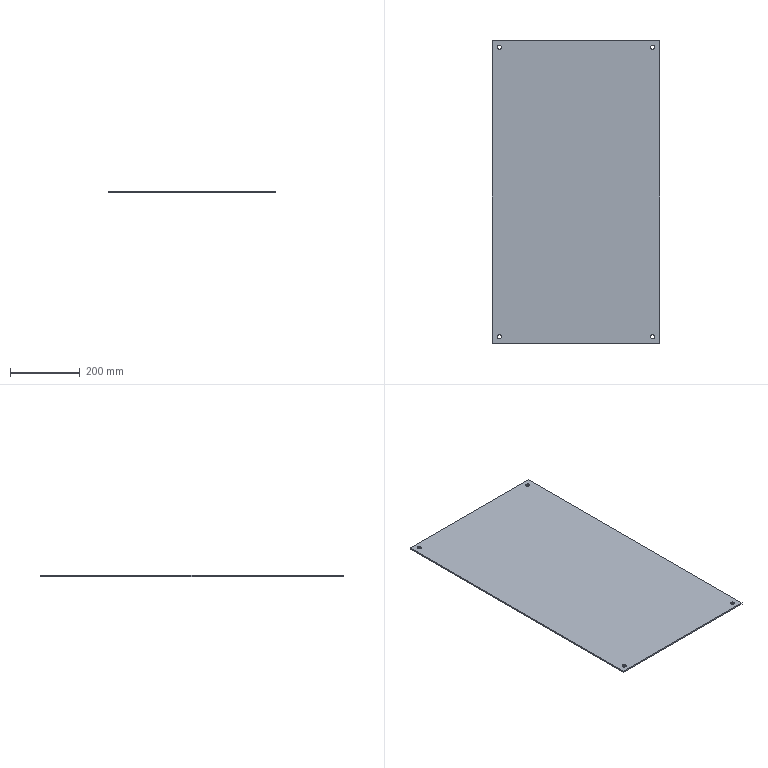Part | STEP file | 02 Middle cover plate | 1 solid | 14 faces | box 480 x 866 x 4 mm | volume 1660910 mm3 | cylinder 8 | plane 6 | commonest cylinder face diameters 12 x8
STEP:
#1=CARTESIAN_POINT('',(0.,0.,0.));
#2=DIRECTION('',(0.,0.,1.));
#3=DIRECTION('',(1.,0.,0.));
#4=AXIS2_PLACEMENT_3D('',#1,#2,#3);
#5=CARTESIAN_POINT('',(14.,-18.,4.));
#6=VERTEX_POINT('',#5);
#7=CARTESIAN_POINT('',(14.,-18.,0.));
#8=VERTEX_POINT('',#7);
#9=CARTESIAN_POINT('',(14.,-18.,4.));
#10=DIRECTION('',(0.,0.,-1.));
#11=VECTOR('',#10,1.);
#12=LINE('',#9,#11);
#13=CARTESIAN_POINT('',(20.,-18.,4.));
#14=DIRECTION('',(0.,0.,-1.));
#15=DIRECTION('',(-1.,0.,0.));
#16=AXIS2_PLACEMENT_3D('',#13,#14,#15);
#17=CYLINDRICAL_SURFACE('',#16,6.);
#18=CARTESIAN_POINT('',(6.283,0.));
#19=DIRECTION('',(0.,1.));
#20=VECTOR('',#19,1.);
#21=LINE('',#18,#20);
#22=(GEOMETRIC_REPRESENTATION_CONTEXT(2)PARAMETRIC_REPRESENTATION_CONTEXT()REPRESENTATION_CONTEXT('',''));
#23=DEFINITIONAL_REPRESENTATION('',(#21),#22);
#24=PCURVE('',#17,#23);
#25=CARTESIAN_POINT('',(20.,-18.,4.));
#26=DIRECTION('',(0.,0.,-1.));
#27=DIRECTION('',(-1.,0.,0.));
#28=AXIS2_PLACEMENT_3D('',#25,#26,#27);
#29=CYLINDRICAL_SURFACE('',#28,6.);
#30=CARTESIAN_POINT('',(0.,0.));
#31=DIRECTION('',(0.,1.));
#32=VECTOR('',#31,1.);
#33=LINE('',#30,#32);
#34=(GEOMETRIC_REPRESENTATION_CONTEXT(2)PARAMETRIC_REPRESENTATION_CONTEXT()REPRESENTATION_CONTEXT('',''));
#35=DEFINITIONAL_REPRESENTATION('',(#33),#34);
#36=PCURVE('',#29,#35);
#37=SURFACE_CURVE('',#12,(#24,#36),.PCURVE_S1.);
#38=EDGE_CURVE('',#6,#8,#37,.T.);
#39=ORIENTED_EDGE('',*,*,#38,.T.);
#40=CARTESIAN_POINT('',(26.,-18.,0.));
#41=VERTEX_POINT('',#40);
#42=CARTESIAN_POINT('',(20.,-18.,0.));
#43=DIRECTION('',(0.,0.,1.));
#44=DIRECTION('',(1.,0.,0.));
#45=AXIS2_PLACEMENT_3D('',#42,#43,#44);
#46=CIRCLE('',#45,6.);
#47=CARTESIAN_POINT('',(9.425,4.));
#48=DIRECTION('',(-1.,0.));
#49=VECTOR('',#48,1.);
#50=LINE('',#47,#49);
#51=(GEOMETRIC_REPRESENTATION_CONTEXT(2)PARAMETRIC_REPRESENTATION_CONTEXT()REPRESENTATION_CONTEXT('',''));
#52=DEFINITIONAL_REPRESENTATION('',(#50),#51);
#53=PCURVE('',#17,#52);
#54=CARTESIAN_POINT('',(0.,0.,0.));
#55=DIRECTION('',(0.,0.,1.));
#56=DIRECTION('',(1.,0.,0.));
#57=AXIS2_PLACEMENT_3D('',#54,#55,#56);
#58=PLANE('',#57);
#59=CARTESIAN_POINT('',(20.,-18.));
#60=DIRECTION('',(1.,0.));
#61=AXIS2_PLACEMENT_2D('',#59,#60);
#62=CIRCLE('',#61,6.);
#63=(GEOMETRIC_REPRESENTATION_CONTEXT(2)PARAMETRIC_REPRESENTATION_CONTEXT()REPRESENTATION_CONTEXT('',''));
#64=DEFINITIONAL_REPRESENTATION('',(#62),#63);
#65=PCURVE('',#58,#64);
#66=SURFACE_CURVE('',#46,(#53,#65),.PCURVE_S1.);
#67=EDGE_CURVE('',#8,#41,#66,.T.);
#68=ORIENTED_EDGE('',*,*,#67,.T.);
#69=CARTESIAN_POINT('',(26.,-18.,4.));
#70=VERTEX_POINT('',#69);
#71=CARTESIAN_POINT('',(26.,-18.,4.));
#72=DIRECTION('',(0.,0.,-1.));
#73=VECTOR('',#72,1.);
#74=LINE('',#71,#73);
#75=CARTESIAN_POINT('',(3.142,0.));
#76=DIRECTION('',(0.,1.));
#77=VECTOR('',#76,1.);
#78=LINE('',#75,#77);
#79=(GEOMETRIC_REPRESENTATION_CONTEXT(2)PARAMETRIC_REPRESENTATION_CONTEXT()REPRESENTATION_CONTEXT('',''));
#80=DEFINITIONAL_REPRESENTATION('',(#78),#79);
#81=PCURVE('',#17,#80);
#82=CARTESIAN_POINT('',(3.142,0.));
#83=DIRECTION('',(0.,1.));
#84=VECTOR('',#83,1.);
#85=LINE('',#82,#84);
#86=(GEOMETRIC_REPRESENTATION_CONTEXT(2)PARAMETRIC_REPRESENTATION_CONTEXT()REPRESENTATION_CONTEXT('',''));
#87=DEFINITIONAL_REPRESENTATION('',(#85),#86);
#88=PCURVE('',#29,#87);
#89=SURFACE_CURVE('',#74,(#81,#88),.PCURVE_S1.);
#90=EDGE_CURVE('',#70,#41,#89,.T.);
#91=ORIENTED_EDGE('',*,*,#90,.F.);
#92=CARTESIAN_POINT('',(20.,-18.,4.));
#93=DIRECTION('',(0.,0.,1.));
#94=DIRECTION('',(1.,0.,0.));
#95=AXIS2_PLACEMENT_3D('',#92,#93,#94);
#96=CIRCLE('',#95,6.);
#97=CARTESIAN_POINT('',(9.425,0.));
#98=DIRECTION('',(-1.,0.));
#99=VECTOR('',#98,1.);
#100=LINE('',#97,#99);
#101=(GEOMETRIC_REPRESENTATION_CONTEXT(2)PARAMETRIC_REPRESENTATION_CONTEXT()REPRESENTATION_CONTEXT('',''));
#102=DEFINITIONAL_REPRESENTATION('',(#100),#101);
#103=PCURVE('',#17,#102);
#104=CARTESIAN_POINT('',(0.,0.,4.));
#105=DIRECTION('',(0.,0.,1.));
#106=DIRECTION('',(1.,0.,0.));
#107=AXIS2_PLACEMENT_3D('',#104,#105,#106);
#108=PLANE('',#107);
#109=CARTESIAN_POINT('',(20.,-18.));
#110=DIRECTION('',(1.,0.));
#111=AXIS2_PLACEMENT_2D('',#109,#110);
#112=CIRCLE('',#111,6.);
#113=(GEOMETRIC_REPRESENTATION_CONTEXT(2)PARAMETRIC_REPRESENTATION_CONTEXT()REPRESENTATION_CONTEXT('',''));
#114=DEFINITIONAL_REPRESENTATION('',(#112),#113);
#115=PCURVE('',#108,#114);
#116=SURFACE_CURVE('',#96,(#103,#115),.PCURVE_S1.);
#117=EDGE_CURVE('',#6,#70,#116,.T.);
#118=ORIENTED_EDGE('',*,*,#117,.F.);
#119=EDGE_LOOP('',(#39,#68,#91,#118));
#120=FACE_BOUND('',#119,.F.);
#121=ADVANCED_FACE('',(#120),#17,.F.);
#122=CARTESIAN_POINT('',(454.,-18.,4.));
#123=VERTEX_POINT('',#122);
#124=CARTESIAN_POINT('',(454.,-18.,0.));
#125=VERTEX_POINT('',#124);
#126=CARTESIAN_POINT('',(454.,-18.,4.));
#127=DIRECTION('',(0.,0.,-1.));
#128=VECTOR('',#127,1.);
#129=LINE('',#126,#128);
#130=CARTESIAN_POINT('',(460.,-18.,4.));
#131=DIRECTION('',(0.,0.,-1.));
#132=DIRECTION('',(-1.,0.,0.));
#133=AXIS2_PLACEMENT_3D('',#130,#131,#132);
#134=CYLINDRICAL_SURFACE('',#133,6.);
#135=CARTESIAN_POINT('',(6.283,0.));
#136=DIRECTION('',(0.,1.));
#137=VECTOR('',#136,1.);
#138=LINE('',#135,#137);
#139=(GEOMETRIC_REPRESENTATION_CONTEXT(2)PARAMETRIC_REPRESENTATION_CONTEXT()REPRESENTATION_CONTEXT('',''));
#140=DEFINITIONAL_REPRESENTATION('',(#138),#139);
#141=PCURVE('',#134,#140);
#142=CARTESIAN_POINT('',(460.,-18.,4.));
#143=DIRECTION('',(0.,0.,-1.));
#144=DIRECTION('',(-1.,0.,0.));
#145=AXIS2_PLACEMENT_3D('',#142,#143,#144);
#146=CYLINDRICAL_SURFACE('',#145,6.);
#147=CARTESIAN_POINT('',(0.,0.));
#148=DIRECTION('',(0.,1.));
#149=VECTOR('',#148,1.);
#150=LINE('',#147,#149);
#151=(GEOMETRIC_REPRESENTATION_CONTEXT(2)PARAMETRIC_REPRESENTATION_CONTEXT()REPRESENTATION_CONTEXT('',''));
#152=DEFINITIONAL_REPRESENTATION('',(#150),#151);
#153=PCURVE('',#146,#152);
#154=SURFACE_CURVE('',#129,(#141,#153),.PCURVE_S1.);
#155=EDGE_CURVE('',#123,#125,#154,.T.);
#156=ORIENTED_EDGE('',*,*,#155,.T.);
#157=CARTESIAN_POINT('',(466.,-18.,0.));
#158=VERTEX_POINT('',#157);
#159=CARTESIAN_POINT('',(460.,-18.,0.));
#160=DIRECTION('',(0.,0.,1.));
#161=DIRECTION('',(1.,0.,0.));
#162=AXIS2_PLACEMENT_3D('',#159,#160,#161);
#163=CIRCLE('',#162,6.);
#164=CARTESIAN_POINT('',(9.425,4.));
#165=DIRECTION('',(-1.,0.));
#166=VECTOR('',#165,1.);
#167=LINE('',#164,#166);
#168=(GEOMETRIC_REPRESENTATION_CONTEXT(2)PARAMETRIC_REPRESENTATION_CONTEXT()REPRESENTATION_CONTEXT('',''));
#169=DEFINITIONAL_REPRESENTATION('',(#167),#168);
#170=PCURVE('',#134,#169);
#171=CARTESIAN_POINT('',(460.,-18.));
#172=DIRECTION('',(1.,0.));
#173=AXIS2_PLACEMENT_2D('',#171,#172);
#174=CIRCLE('',#173,6.);
#175=(GEOMETRIC_REPRESENTATION_CONTEXT(2)PARAMETRIC_REPRESENTATION_CONTEXT()REPRESENTATION_CONTEXT('',''));
#176=DEFINITIONAL_REPRESENTATION('',(#174),#175);
#177=PCURVE('',#58,#176);
#178=SURFACE_CURVE('',#163,(#170,#177),.PCURVE_S1.);
#179=EDGE_CURVE('',#125,#158,#178,.T.);
#180=ORIENTED_EDGE('',*,*,#179,.T.);
#181=CARTESIAN_POINT('',(466.,-18.,4.));
#182=VERTEX_POINT('',#181);
#183=CARTESIAN_POINT('',(466.,-18.,4.));
#184=DIRECTION('',(0.,0.,-1.));
#185=VECTOR('',#184,1.);
#186=LINE('',#183,#185);
#187=CARTESIAN_POINT('',(3.142,0.));
#188=DIRECTION('',(0.,1.));
#189=VECTOR('',#188,1.);
#190=LINE('',#187,#189);
#191=(GEOMETRIC_REPRESENTATION_CONTEXT(2)PARAMETRIC_REPRESENTATION_CONTEXT()REPRESENTATION_CONTEXT('',''));
#192=DEFINITIONAL_REPRESENTATION('',(#190),#191);
#193=PCURVE('',#134,#192);
#194=CARTESIAN_POINT('',(3.142,0.));
#195=DIRECTION('',(0.,1.));
#196=VECTOR('',#195,1.);
#197=LINE('',#194,#196);
#198=(GEOMETRIC_REPRESENTATION_CONTEXT(2)PARAMETRIC_REPRESENTATION_CONTEXT()REPRESENTATION_CONTEXT('',''));
#199=DEFINITIONAL_REPRESENTATION('',(#197),#198);
#200=PCURVE('',#146,#199);
#201=SURFACE_CURVE('',#186,(#193,#200),.PCURVE_S1.);
#202=EDGE_CURVE('',#182,#158,#201,.T.);
#203=ORIENTED_EDGE('',*,*,#202,.F.);
#204=CARTESIAN_POINT('',(460.,-18.,4.));
#205=DIRECTION('',(0.,0.,1.));
#206=DIRECTION('',(1.,0.,0.));
#207=AXIS2_PLACEMENT_3D('',#204,#205,#206);
#208=CIRCLE('',#207,6.);
#209=CARTESIAN_POINT('',(9.425,0.));
#210=DIRECTION('',(-1.,0.));
#211=VECTOR('',#210,1.);
#212=LINE('',#209,#211);
#213=(GEOMETRIC_REPRESENTATION_CONTEXT(2)PARAMETRIC_REPRESENTATION_CONTEXT()REPRESENTATION_CONTEXT('',''));
#214=DEFINITIONAL_REPRESENTATION('',(#212),#213);
#215=PCURVE('',#134,#214);
#216=CARTESIAN_POINT('',(460.,-18.));
#217=DIRECTION('',(1.,0.));
#218=AXIS2_PLACEMENT_2D('',#216,#217);
#219=CIRCLE('',#218,6.);
#220=(GEOMETRIC_REPRESENTATION_CONTEXT(2)PARAMETRIC_REPRESENTATION_CONTEXT()REPRESENTATION_CONTEXT('',''));
#221=DEFINITIONAL_REPRESENTATION('',(#219),#220);
#222=PCURVE('',#108,#221);
#223=SURFACE_CURVE('',#208,(#215,#222),.PCURVE_S1.);
#224=EDGE_CURVE('',#123,#182,#223,.T.);
#225=ORIENTED_EDGE('',*,*,#224,.F.);
#226=EDGE_LOOP('',(#156,#180,#203,#225));
#227=FACE_BOUND('',#226,.F.);
#228=ADVANCED_FACE('',(#227),#134,.F.);
#229=CARTESIAN_POINT('',(454.,-848.,4.));
#230=VERTEX_POINT('',#229);
#231=CARTESIAN_POINT('',(454.,-848.,0.));
#232=VERTEX_POINT('',#231);
#233=CARTESIAN_POINT('',(454.,-848.,4.));
#234=DIRECTION('',(0.,0.,-1.));
#235=VECTOR('',#234,1.);
#236=LINE('',#233,#235);
#237=CARTESIAN_POINT('',(460.,-848.,4.));
#238=DIRECTION('',(0.,0.,-1.));
#239=DIRECTION('',(-1.,0.,0.));
#240=AXIS2_PLACEMENT_3D('',#237,#238,#239);
#241=CYLINDRICAL_SURFACE('',#240,6.);
#242=CARTESIAN_POINT('',(6.283,0.));
#243=DIRECTION('',(0.,1.));
#244=VECTOR('',#243,1.);
#245=LINE('',#242,#244);
#246=(GEOMETRIC_REPRESENTATION_CONTEXT(2)PARAMETRIC_REPRESENTATION_CONTEXT()REPRESENTATION_CONTEXT('',''));
#247=DEFINITIONAL_REPRESENTATION('',(#245),#246);
#248=PCURVE('',#241,#247);
#249=CARTESIAN_POINT('',(460.,-848.,4.));
#250=DIRECTION('',(0.,0.,-1.));
#251=DIRECTION('',(-1.,0.,0.));
#252=AXIS2_PLACEMENT_3D('',#249,#250,#251);
#253=CYLINDRICAL_SURFACE('',#252,6.);
#254=CARTESIAN_POINT('',(0.,0.));
#255=DIRECTION('',(0.,1.));
#256=VECTOR('',#255,1.);
#257=LINE('',#254,#256);
#258=(GEOMETRIC_REPRESENTATION_CONTEXT(2)PARAMETRIC_REPRESENTATION_CONTEXT()REPRESENTATION_CONTEXT('',''));
#259=DEFINITIONAL_REPRESENTATION('',(#257),#258);
#260=PCURVE('',#253,#259);
#261=SURFACE_CURVE('',#236,(#248,#260),.PCURVE_S1.);
#262=EDGE_CURVE('',#230,#232,#261,.T.);
#263=ORIENTED_EDGE('',*,*,#262,.T.);
#264=CARTESIAN_POINT('',(466.,-848.,0.));
#265=VERTEX_POINT('',#264);
#266=CARTESIAN_POINT('',(460.,-848.,0.));
#267=DIRECTION('',(0.,0.,1.));
#268=DIRECTION('',(1.,0.,0.));
#269=AXIS2_PLACEMENT_3D('',#266,#267,#268);
#270=CIRCLE('',#269,6.);
#271=CARTESIAN_POINT('',(9.425,4.));
#272=DIRECTION('',(-1.,0.));
#273=VECTOR('',#272,1.);
#274=LINE('',#271,#273);
#275=(GEOMETRIC_REPRESENTATION_CONTEXT(2)PARAMETRIC_REPRESENTATION_CONTEXT()REPRESENTATION_CONTEXT('',''));
#276=DEFINITIONAL_REPRESENTATION('',(#274),#275);
#277=PCURVE('',#241,#276);
#278=CARTESIAN_POINT('',(460.,-848.));
#279=DIRECTION('',(1.,0.));
#280=AXIS2_PLACEMENT_2D('',#278,#279);
#281=CIRCLE('',#280,6.);
#282=(GEOMETRIC_REPRESENTATION_CONTEXT(2)PARAMETRIC_REPRESENTATION_CONTEXT()REPRESENTATION_CONTEXT('',''));
#283=DEFINITIONAL_REPRESENTATION('',(#281),#282);
#284=PCURVE('',#58,#283);
#285=SURFACE_CURVE('',#270,(#277,#284),.PCURVE_S1.);
#286=EDGE_CURVE('',#232,#265,#285,.T.);
#287=ORIENTED_EDGE('',*,*,#286,.T.);
#288=CARTESIAN_POINT('',(466.,-848.,4.));
#289=VERTEX_POINT('',#288);
#290=CARTESIAN_POINT('',(466.,-848.,4.));
#291=DIRECTION('',(0.,0.,-1.));
#292=VECTOR('',#291,1.);
#293=LINE('',#290,#292);
#294=CARTESIAN_POINT('',(3.142,0.));
#295=DIRECTION('',(0.,1.));
#296=VECTOR('',#295,1.);
#297=LINE('',#294,#296);
#298=(GEOMETRIC_REPRESENTATION_CONTEXT(2)PARAMETRIC_REPRESENTATION_CONTEXT()REPRESENTATION_CONTEXT('',''));
#299=DEFINITIONAL_REPRESENTATION('',(#297),#298);
#300=PCURVE('',#241,#299);
#301=CARTESIAN_POINT('',(3.142,0.));
#302=DIRECTION('',(0.,1.));
#303=VECTOR('',#302,1.);
#304=LINE('',#301,#303);
#305=(GEOMETRIC_REPRESENTATION_CONTEXT(2)PARAMETRIC_REPRESENTATION_CONTEXT()REPRESENTATION_CONTEXT('',''));
#306=DEFINITIONAL_REPRESENTATION('',(#304),#305);
#307=PCURVE('',#253,#306);
#308=SURFACE_CURVE('',#293,(#300,#307),.PCURVE_S1.);
#309=EDGE_CURVE('',#289,#265,#308,.T.);
#310=ORIENTED_EDGE('',*,*,#309,.F.);
#311=CARTESIAN_POINT('',(460.,-848.,4.));
#312=DIRECTION('',(0.,0.,1.));
#313=DIRECTION('',(1.,0.,0.));
#314=AXIS2_PLACEMENT_3D('',#311,#312,#313);
#315=CIRCLE('',#314,6.);
#316=CARTESIAN_POINT('',(9.425,0.));
#317=DIRECTION('',(-1.,0.));
#318=VECTOR('',#317,1.);
#319=LINE('',#316,#318);
#320=(GEOMETRIC_REPRESENTATION_CONTEXT(2)PARAMETRIC_REPRESENTATION_CONTEXT()REPRESENTATION_CONTEXT('',''));
#321=DEFINITIONAL_REPRESENTATION('',(#319),#320);
#322=PCURVE('',#241,#321);
#323=CARTESIAN_POINT('',(460.,-848.));
#324=DIRECTION('',(1.,0.));
#325=AXIS2_PLACEMENT_2D('',#323,#324);
#326=CIRCLE('',#325,6.);
#327=(GEOMETRIC_REPRESENTATION_CONTEXT(2)PARAMETRIC_REPRESENTATION_CONTEXT()REPRESENTATION_CONTEXT('',''));
#328=DEFINITIONAL_REPRESENTATION('',(#326),#327);
#329=PCURVE('',#108,#328);
#330=SURFACE_CURVE('',#315,(#322,#329),.PCURVE_S1.);
#331=EDGE_CURVE('',#230,#289,#330,.T.);
#332=ORIENTED_EDGE('',*,*,#331,.F.);
#333=EDGE_LOOP('',(#263,#287,#310,#332));
#334=FACE_BOUND('',#333,.F.);
#335=ADVANCED_FACE('',(#334),#241,.F.);
#336=CARTESIAN_POINT('',(14.,-848.,4.));
#337=VERTEX_POINT('',#336);
#338=CARTESIAN_POINT('',(14.,-848.,0.));
#339=VERTEX_POINT('',#338);
#340=CARTESIAN_POINT('',(14.,-848.,4.));
#341=DIRECTION('',(0.,0.,-1.));
#342=VECTOR('',#341,1.);
#343=LINE('',#340,#342);
#344=CARTESIAN_POINT('',(20.,-848.,4.));
#345=DIRECTION('',(0.,0.,-1.));
#346=DIRECTION('',(-1.,0.,0.));
#347=AXIS2_PLACEMENT_3D('',#344,#345,#346);
#348=CYLINDRICAL_SURFACE('',#347,6.);
#349=CARTESIAN_POINT('',(6.283,0.));
#350=DIRECTION('',(0.,1.));
#351=VECTOR('',#350,1.);
#352=LINE('',#349,#351);
#353=(GEOMETRIC_REPRESENTATION_CONTEXT(2)PARAMETRIC_REPRESENTATION_CONTEXT()REPRESENTATION_CONTEXT('',''));
#354=DEFINITIONAL_REPRESENTATION('',(#352),#353);
#355=PCURVE('',#348,#354);
#356=CARTESIAN_POINT('',(20.,-848.,4.));
#357=DIRECTION('',(0.,0.,-1.));
#358=DIRECTION('',(-1.,0.,0.));
#359=AXIS2_PLACEMENT_3D('',#356,#357,#358);
#360=CYLINDRICAL_SURFACE('',#359,6.);
#361=CARTESIAN_POINT('',(0.,0.));
#362=DIRECTION('',(0.,1.));
#363=VECTOR('',#362,1.);
#364=LINE('',#361,#363);
#365=(GEOMETRIC_REPRESENTATION_CONTEXT(2)PARAMETRIC_REPRESENTATION_CONTEXT()REPRESENTATION_CONTEXT('',''));
#366=DEFINITIONAL_REPRESENTATION('',(#364),#365);
#367=PCURVE('',#360,#366);
#368=SURFACE_CURVE('',#343,(#355,#367),.PCURVE_S1.);
#369=EDGE_CURVE('',#337,#339,#368,.T.);
#370=ORIENTED_EDGE('',*,*,#369,.T.);
#371=CARTESIAN_POINT('',(26.,-848.,0.));
#372=VERTEX_POINT('',#371);
#373=CARTESIAN_POINT('',(20.,-848.,0.));
#374=DIRECTION('',(0.,0.,1.));
#375=DIRECTION('',(1.,0.,0.));
#376=AXIS2_PLACEMENT_3D('',#373,#374,#375);
#377=CIRCLE('',#376,6.);
#378=CARTESIAN_POINT('',(9.425,4.));
#379=DIRECTION('',(-1.,0.));
#380=VECTOR('',#379,1.);
#381=LINE('',#378,#380);
#382=(GEOMETRIC_REPRESENTATION_CONTEXT(2)PARAMETRIC_REPRESENTATION_CONTEXT()REPRESENTATION_CONTEXT('',''));
#383=DEFINITIONAL_REPRESENTATION('',(#381),#382);
#384=PCURVE('',#348,#383);
#385=CARTESIAN_POINT('',(20.,-848.));
#386=DIRECTION('',(1.,0.));
#387=AXIS2_PLACEMENT_2D('',#385,#386);
#388=CIRCLE('',#387,6.);
#389=(GEOMETRIC_REPRESENTATION_CONTEXT(2)PARAMETRIC_REPRESENTATION_CONTEXT()REPRESENTATION_CONTEXT('',''));
#390=DEFINITIONAL_REPRESENTATION('',(#388),#389);
#391=PCURVE('',#58,#390);
#392=SURFACE_CURVE('',#377,(#384,#391),.PCURVE_S1.);
#393=EDGE_CURVE('',#339,#372,#392,.T.);
#394=ORIENTED_EDGE('',*,*,#393,.T.);
#395=CARTESIAN_POINT('',(26.,-848.,4.));
#396=VERTEX_POINT('',#395);
#397=CARTESIAN_POINT('',(26.,-848.,4.));
#398=DIRECTION('',(0.,0.,-1.));
#399=VECTOR('',#398,1.);
#400=LINE('',#397,#399);
#401=CARTESIAN_POINT('',(3.142,0.));
#402=DIRECTION('',(0.,1.));
#403=VECTOR('',#402,1.);
#404=LINE('',#401,#403);
#405=(GEOMETRIC_REPRESENTATION_CONTEXT(2)PARAMETRIC_REPRESENTATION_CONTEXT()REPRESENTATION_CONTEXT('',''));
#406=DEFINITIONAL_REPRESENTATION('',(#404),#405);
#407=PCURVE('',#348,#406);
#408=CARTESIAN_POINT('',(3.142,0.));
#409=DIRECTION('',(0.,1.));
#410=VECTOR('',#409,1.);
#411=LINE('',#408,#410);
#412=(GEOMETRIC_REPRESENTATION_CONTEXT(2)PARAMETRIC_REPRESENTATION_CONTEXT()REPRESENTATION_CONTEXT('',''));
#413=DEFINITIONAL_REPRESENTATION('',(#411),#412);
#414=PCURVE('',#360,#413);
#415=SURFACE_CURVE('',#400,(#407,#414),.PCURVE_S1.);
#416=EDGE_CURVE('',#396,#372,#415,.T.);
#417=ORIENTED_EDGE('',*,*,#416,.F.);
#418=CARTESIAN_POINT('',(20.,-848.,4.));
#419=DIRECTION('',(0.,0.,1.));
#420=DIRECTION('',(1.,0.,0.));
#421=AXIS2_PLACEMENT_3D('',#418,#419,#420);
#422=CIRCLE('',#421,6.);
#423=CARTESIAN_POINT('',(9.425,0.));
#424=DIRECTION('',(-1.,0.));
#425=VECTOR('',#424,1.);
#426=LINE('',#423,#425);
#427=(GEOMETRIC_REPRESENTATION_CONTEXT(2)PARAMETRIC_REPRESENTATION_CONTEXT()REPRESENTATION_CONTEXT('',''));
#428=DEFINITIONAL_REPRESENTATION('',(#426),#427);
#429=PCURVE('',#348,#428);
#430=CARTESIAN_POINT('',(20.,-848.));
#431=DIRECTION('',(1.,0.));
#432=AXIS2_PLACEMENT_2D('',#430,#431);
#433=CIRCLE('',#432,6.);
#434=(GEOMETRIC_REPRESENTATION_CONTEXT(2)PARAMETRIC_REPRESENTATION_CONTEXT()REPRESENTATION_CONTEXT('',''));
#435=DEFINITIONAL_REPRESENTATION('',(#433),#434);
#436=PCURVE('',#108,#435);
#437=SURFACE_CURVE('',#422,(#429,#436),.PCURVE_S1.);
#438=EDGE_CURVE('',#337,#396,#437,.T.);
#439=ORIENTED_EDGE('',*,*,#438,.F.);
#440=EDGE_LOOP('',(#370,#394,#417,#439));
#441=FACE_BOUND('',#440,.F.);
#442=ADVANCED_FACE('',(#441),#348,.F.);
#443=ORIENTED_EDGE('',*,*,#224,.F.);
#444=CARTESIAN_POINT('',(460.,-18.,4.));
#445=DIRECTION('',(0.,0.,1.));
#446=DIRECTION('',(1.,0.,0.));
#447=AXIS2_PLACEMENT_3D('',#444,#445,#446);
#448=CIRCLE('',#447,6.);
#449=CARTESIAN_POINT('',(460.,-18.));
#450=DIRECTION('',(1.,0.));
#451=AXIS2_PLACEMENT_2D('',#449,#450);
#452=CIRCLE('',#451,6.);
#453=(GEOMETRIC_REPRESENTATION_CONTEXT(2)PARAMETRIC_REPRESENTATION_CONTEXT()REPRESENTATION_CONTEXT('',''));
#454=DEFINITIONAL_REPRESENTATION('',(#452),#453);
#455=PCURVE('',#108,#454);
#456=CARTESIAN_POINT('',(3.142,0.));
#457=DIRECTION('',(-1.,0.));
#458=VECTOR('',#457,1.);
#459=LINE('',#456,#458);
#460=(GEOMETRIC_REPRESENTATION_CONTEXT(2)PARAMETRIC_REPRESENTATION_CONTEXT()REPRESENTATION_CONTEXT('',''));
#461=DEFINITIONAL_REPRESENTATION('',(#459),#460);
#462=PCURVE('',#146,#461);
#463=SURFACE_CURVE('',#448,(#455,#462),.PCURVE_S1.);
#464=EDGE_CURVE('',#182,#123,#463,.T.);
#465=ORIENTED_EDGE('',*,*,#464,.F.);
#466=EDGE_LOOP('',(#443,#465));
#467=FACE_BOUND('',#466,.T.);
#468=ORIENTED_EDGE('',*,*,#438,.F.);
#469=CARTESIAN_POINT('',(20.,-848.,4.));
#470=DIRECTION('',(0.,0.,1.));
#471=DIRECTION('',(1.,0.,0.));
#472=AXIS2_PLACEMENT_3D('',#469,#470,#471);
#473=CIRCLE('',#472,6.);
#474=CARTESIAN_POINT('',(20.,-848.));
#475=DIRECTION('',(1.,0.));
#476=AXIS2_PLACEMENT_2D('',#474,#475);
#477=CIRCLE('',#476,6.);
#478=(GEOMETRIC_REPRESENTATION_CONTEXT(2)PARAMETRIC_REPRESENTATION_CONTEXT()REPRESENTATION_CONTEXT('',''));
#479=DEFINITIONAL_REPRESENTATION('',(#477),#478);
#480=PCURVE('',#108,#479);
#481=CARTESIAN_POINT('',(3.142,0.));
#482=DIRECTION('',(-1.,0.));
#483=VECTOR('',#482,1.);
#484=LINE('',#481,#483);
#485=(GEOMETRIC_REPRESENTATION_CONTEXT(2)PARAMETRIC_REPRESENTATION_CONTEXT()REPRESENTATION_CONTEXT('',''));
#486=DEFINITIONAL_REPRESENTATION('',(#484),#485);
#487=PCURVE('',#360,#486);
#488=SURFACE_CURVE('',#473,(#480,#487),.PCURVE_S1.);
#489=EDGE_CURVE('',#396,#337,#488,.T.);
#490=ORIENTED_EDGE('',*,*,#489,.F.);
#491=EDGE_LOOP('',(#468,#490));
#492=FACE_BOUND('',#491,.T.);
#493=CARTESIAN_POINT('',(0.,0.,4.));
#494=VERTEX_POINT('',#493);
#495=CARTESIAN_POINT('',(0.,-866.,4.));
#496=VERTEX_POINT('',#495);
#497=CARTESIAN_POINT('',(0.,0.,4.));
#498=DIRECTION('',(0.,-1.,0.));
#499=VECTOR('',#498,1.);
#500=LINE('',#497,#499);
#501=CARTESIAN_POINT('',(0.,0.));
#502=DIRECTION('',(0.,-1.));
#503=VECTOR('',#502,1.);
#504=LINE('',#501,#503);
#505=(GEOMETRIC_REPRESENTATION_CONTEXT(2)PARAMETRIC_REPRESENTATION_CONTEXT()REPRESENTATION_CONTEXT('',''));
#506=DEFINITIONAL_REPRESENTATION('',(#504),#505);
#507=PCURVE('',#108,#506);
#508=CARTESIAN_POINT('',(0.,0.,4.));
#509=DIRECTION('',(1.,0.,0.));
#510=DIRECTION('',(0.,1.,0.));
#511=AXIS2_PLACEMENT_3D('',#508,#509,#510);
#512=PLANE('',#511);
#513=CARTESIAN_POINT('',(0.,0.));
#514=DIRECTION('',(-1.,0.));
#515=VECTOR('',#514,1.);
#516=LINE('',#513,#515);
#517=(GEOMETRIC_REPRESENTATION_CONTEXT(2)PARAMETRIC_REPRESENTATION_CONTEXT()REPRESENTATION_CONTEXT('',''));
#518=DEFINITIONAL_REPRESENTATION('',(#516),#517);
#519=PCURVE('',#512,#518);
#520=SURFACE_CURVE('',#500,(#507,#519),.PCURVE_S1.);
#521=EDGE_CURVE('',#494,#496,#520,.T.);
#522=ORIENTED_EDGE('',*,*,#521,.T.);
#523=CARTESIAN_POINT('',(480.,-866.,4.));
#524=VERTEX_POINT('',#523);
#525=CARTESIAN_POINT('',(0.,-866.,4.));
#526=DIRECTION('',(1.,0.,0.));
#527=VECTOR('',#526,1.);
#528=LINE('',#525,#527);
#529=CARTESIAN_POINT('',(0.,-866.));
#530=DIRECTION('',(1.,0.));
#531=VECTOR('',#530,1.);
#532=LINE('',#529,#531);
#533=(GEOMETRIC_REPRESENTATION_CONTEXT(2)PARAMETRIC_REPRESENTATION_CONTEXT()REPRESENTATION_CONTEXT('',''));
#534=DEFINITIONAL_REPRESENTATION('',(#532),#533);
#535=PCURVE('',#108,#534);
#536=CARTESIAN_POINT('',(0.,-866.,4.));
#537=DIRECTION('',(0.,1.,0.));
#538=DIRECTION('',(0.,0.,1.));
#539=AXIS2_PLACEMENT_3D('',#536,#537,#538);
#540=PLANE('',#539);
#541=CARTESIAN_POINT('',(0.,0.));
#542=DIRECTION('',(0.,1.));
#543=VECTOR('',#542,1.);
#544=LINE('',#541,#543);
#545=(GEOMETRIC_REPRESENTATION_CONTEXT(2)PARAMETRIC_REPRESENTATION_CONTEXT()REPRESENTATION_CONTEXT('',''));
#546=DEFINITIONAL_REPRESENTATION('',(#544),#545);
#547=PCURVE('',#540,#546);
#548=SURFACE_CURVE('',#528,(#535,#547),.PCURVE_S1.);
#549=EDGE_CURVE('',#496,#524,#548,.T.);
#550=ORIENTED_EDGE('',*,*,#549,.T.);
#551=CARTESIAN_POINT('',(480.,0.,4.));
#552=VERTEX_POINT('',#551);
#553=CARTESIAN_POINT('',(480.,0.,4.));
#554=DIRECTION('',(0.,1.,0.));
#555=VECTOR('',#554,1.);
#556=LINE('',#553,#555);
#557=CARTESIAN_POINT('',(480.,0.));
#558=DIRECTION('',(0.,1.));
#559=VECTOR('',#558,1.);
#560=LINE('',#557,#559);
#561=(GEOMETRIC_REPRESENTATION_CONTEXT(2)PARAMETRIC_REPRESENTATION_CONTEXT()REPRESENTATION_CONTEXT('',''));
#562=DEFINITIONAL_REPRESENTATION('',(#560),#561);
#563=PCURVE('',#108,#562);
#564=CARTESIAN_POINT('',(480.,0.,4.));
#565=DIRECTION('',(-1.,0.,0.));
#566=DIRECTION('',(0.,0.,1.));
#567=AXIS2_PLACEMENT_3D('',#564,#565,#566);
#568=PLANE('',#567);
#569=CARTESIAN_POINT('',(0.,0.));
#570=DIRECTION('',(0.,1.));
#571=VECTOR('',#570,1.);
#572=LINE('',#569,#571);
#573=(GEOMETRIC_REPRESENTATION_CONTEXT(2)PARAMETRIC_REPRESENTATION_CONTEXT()REPRESENTATION_CONTEXT('',''));
#574=DEFINITIONAL_REPRESENTATION('',(#572),#573);
#575=PCURVE('',#568,#574);
#576=SURFACE_CURVE('',#556,(#563,#575),.PCURVE_S1.);
#577=EDGE_CURVE('',#524,#552,#576,.T.);
#578=ORIENTED_EDGE('',*,*,#577,.T.);
#579=CARTESIAN_POINT('',(0.,0.,4.));
#580=DIRECTION('',(-1.,0.,0.));
#581=VECTOR('',#580,1.);
#582=LINE('',#579,#581);
#583=CARTESIAN_POINT('',(0.,0.));
#584=DIRECTION('',(-1.,0.));
#585=VECTOR('',#584,1.);
#586=LINE('',#583,#585);
#587=(GEOMETRIC_REPRESENTATION_CONTEXT(2)PARAMETRIC_REPRESENTATION_CONTEXT()REPRESENTATION_CONTEXT('',''));
#588=DEFINITIONAL_REPRESENTATION('',(#586),#587);
#589=PCURVE('',#108,#588);
#590=CARTESIAN_POINT('',(0.,0.,4.));
#591=DIRECTION('',(0.,-1.,0.));
#592=DIRECTION('',(1.,0.,0.));
#593=AXIS2_PLACEMENT_3D('',#590,#591,#592);
#594=PLANE('',#593);
#595=CARTESIAN_POINT('',(0.,0.));
#596=DIRECTION('',(-1.,0.));
#597=VECTOR('',#596,1.);
#598=LINE('',#595,#597);
#599=(GEOMETRIC_REPRESENTATION_CONTEXT(2)PARAMETRIC_REPRESENTATION_CONTEXT()REPRESENTATION_CONTEXT('',''));
#600=DEFINITIONAL_REPRESENTATION('',(#598),#599);
#601=PCURVE('',#594,#600);
#602=SURFACE_CURVE('',#582,(#589,#601),.PCURVE_S1.);
#603=EDGE_CURVE('',#552,#494,#602,.T.);
#604=ORIENTED_EDGE('',*,*,#603,.T.);
#605=EDGE_LOOP('',(#522,#550,#578,#604));
#606=FACE_BOUND('',#605,.T.);
#607=ORIENTED_EDGE('',*,*,#331,.F.);
#608=CARTESIAN_POINT('',(460.,-848.,4.));
#609=DIRECTION('',(0.,0.,1.));
#610=DIRECTION('',(1.,0.,0.));
#611=AXIS2_PLACEMENT_3D('',#608,#609,#610);
#612=CIRCLE('',#611,6.);
#613=CARTESIAN_POINT('',(460.,-848.));
#614=DIRECTION('',(1.,0.));
#615=AXIS2_PLACEMENT_2D('',#613,#614);
#616=CIRCLE('',#615,6.);
#617=(GEOMETRIC_REPRESENTATION_CONTEXT(2)PARAMETRIC_REPRESENTATION_CONTEXT()REPRESENTATION_CONTEXT('',''));
#618=DEFINITIONAL_REPRESENTATION('',(#616),#617);
#619=PCURVE('',#108,#618);
#620=CARTESIAN_POINT('',(3.142,0.));
#621=DIRECTION('',(-1.,0.));
#622=VECTOR('',#621,1.);
#623=LINE('',#620,#622);
#624=(GEOMETRIC_REPRESENTATION_CONTEXT(2)PARAMETRIC_REPRESENTATION_CONTEXT()REPRESENTATION_CONTEXT('',''));
#625=DEFINITIONAL_REPRESENTATION('',(#623),#624);
#626=PCURVE('',#253,#625);
#627=SURFACE_CURVE('',#612,(#619,#626),.PCURVE_S1.);
#628=EDGE_CURVE('',#289,#230,#627,.T.);
#629=ORIENTED_EDGE('',*,*,#628,.F.);
#630=EDGE_LOOP('',(#607,#629));
#631=FACE_BOUND('',#630,.T.);
#632=ORIENTED_EDGE('',*,*,#117,.F.);
#633=CARTESIAN_POINT('',(20.,-18.,4.));
#634=DIRECTION('',(0.,0.,1.));
#635=DIRECTION('',(1.,0.,0.));
#636=AXIS2_PLACEMENT_3D('',#633,#634,#635);
#637=CIRCLE('',#636,6.);
#638=CARTESIAN_POINT('',(20.,-18.));
#639=DIRECTION('',(1.,0.));
#640=AXIS2_PLACEMENT_2D('',#638,#639);
#641=CIRCLE('',#640,6.);
#642=(GEOMETRIC_REPRESENTATION_CONTEXT(2)PARAMETRIC_REPRESENTATION_CONTEXT()REPRESENTATION_CONTEXT('',''));
#643=DEFINITIONAL_REPRESENTATION('',(#641),#642);
#644=PCURVE('',#108,#643);
#645=CARTESIAN_POINT('',(3.142,0.));
#646=DIRECTION('',(-1.,0.));
#647=VECTOR('',#646,1.);
#648=LINE('',#645,#647);
#649=(GEOMETRIC_REPRESENTATION_CONTEXT(2)PARAMETRIC_REPRESENTATION_CONTEXT()REPRESENTATION_CONTEXT('',''));
#650=DEFINITIONAL_REPRESENTATION('',(#648),#649);
#651=PCURVE('',#29,#650);
#652=SURFACE_CURVE('',#637,(#644,#651),.PCURVE_S1.);
#653=EDGE_CURVE('',#70,#6,#652,.T.);
#654=ORIENTED_EDGE('',*,*,#653,.F.);
#655=EDGE_LOOP('',(#632,#654));
#656=FACE_BOUND('',#655,.T.);
#657=ADVANCED_FACE('',(#467,#492,#606,#631,#656),#108,.T.);
#658=ORIENTED_EDGE('',*,*,#179,.T.);
#659=CARTESIAN_POINT('',(460.,-18.,0.));
#660=DIRECTION('',(0.,0.,1.));
#661=DIRECTION('',(1.,0.,0.));
#662=AXIS2_PLACEMENT_3D('',#659,#660,#661);
#663=CIRCLE('',#662,6.);
#664=CARTESIAN_POINT('',(460.,-18.));
#665=DIRECTION('',(1.,0.));
#666=AXIS2_PLACEMENT_2D('',#664,#665);
#667=CIRCLE('',#666,6.);
#668=(GEOMETRIC_REPRESENTATION_CONTEXT(2)PARAMETRIC_REPRESENTATION_CONTEXT()REPRESENTATION_CONTEXT('',''));
#669=DEFINITIONAL_REPRESENTATION('',(#667),#668);
#670=PCURVE('',#58,#669);
#671=CARTESIAN_POINT('',(3.142,4.));
#672=DIRECTION('',(-1.,0.));
#673=VECTOR('',#672,1.);
#674=LINE('',#671,#673);
#675=(GEOMETRIC_REPRESENTATION_CONTEXT(2)PARAMETRIC_REPRESENTATION_CONTEXT()REPRESENTATION_CONTEXT('',''));
#676=DEFINITIONAL_REPRESENTATION('',(#674),#675);
#677=PCURVE('',#146,#676);
#678=SURFACE_CURVE('',#663,(#670,#677),.PCURVE_S1.);
#679=EDGE_CURVE('',#158,#125,#678,.T.);
#680=ORIENTED_EDGE('',*,*,#679,.T.);
#681=EDGE_LOOP('',(#658,#680));
#682=FACE_BOUND('',#681,.T.);
#683=ORIENTED_EDGE('',*,*,#393,.T.);
#684=CARTESIAN_POINT('',(20.,-848.,0.));
#685=DIRECTION('',(0.,0.,1.));
#686=DIRECTION('',(1.,0.,0.));
#687=AXIS2_PLACEMENT_3D('',#684,#685,#686);
#688=CIRCLE('',#687,6.);
#689=CARTESIAN_POINT('',(20.,-848.));
#690=DIRECTION('',(1.,0.));
#691=AXIS2_PLACEMENT_2D('',#689,#690);
#692=CIRCLE('',#691,6.);
#693=(GEOMETRIC_REPRESENTATION_CONTEXT(2)PARAMETRIC_REPRESENTATION_CONTEXT()REPRESENTATION_CONTEXT('',''));
#694=DEFINITIONAL_REPRESENTATION('',(#692),#693);
#695=PCURVE('',#58,#694);
#696=CARTESIAN_POINT('',(3.142,4.));
#697=DIRECTION('',(-1.,0.));
#698=VECTOR('',#697,1.);
#699=LINE('',#696,#698);
#700=(GEOMETRIC_REPRESENTATION_CONTEXT(2)PARAMETRIC_REPRESENTATION_CONTEXT()REPRESENTATION_CONTEXT('',''));
#701=DEFINITIONAL_REPRESENTATION('',(#699),#700);
#702=PCURVE('',#360,#701);
#703=SURFACE_CURVE('',#688,(#695,#702),.PCURVE_S1.);
#704=EDGE_CURVE('',#372,#339,#703,.T.);
#705=ORIENTED_EDGE('',*,*,#704,.T.);
#706=EDGE_LOOP('',(#683,#705));
#707=FACE_BOUND('',#706,.T.);
#708=CARTESIAN_POINT('',(0.,0.,0.));
#709=VERTEX_POINT('',#708);
#710=CARTESIAN_POINT('',(0.,-866.,0.));
#711=VERTEX_POINT('',#710);
#712=CARTESIAN_POINT('',(0.,0.,0.));
#713=DIRECTION('',(0.,-1.,0.));
#714=VECTOR('',#713,1.);
#715=LINE('',#712,#714);
#716=CARTESIAN_POINT('',(0.,0.));
#717=DIRECTION('',(0.,-1.));
#718=VECTOR('',#717,1.);
#719=LINE('',#716,#718);
#720=(GEOMETRIC_REPRESENTATION_CONTEXT(2)PARAMETRIC_REPRESENTATION_CONTEXT()REPRESENTATION_CONTEXT('',''));
#721=DEFINITIONAL_REPRESENTATION('',(#719),#720);
#722=PCURVE('',#58,#721);
#723=CARTESIAN_POINT('',(0.,-4.));
#724=DIRECTION('',(-1.,0.));
#725=VECTOR('',#724,1.);
#726=LINE('',#723,#725);
#727=(GEOMETRIC_REPRESENTATION_CONTEXT(2)PARAMETRIC_REPRESENTATION_CONTEXT()REPRESENTATION_CONTEXT('',''));
#728=DEFINITIONAL_REPRESENTATION('',(#726),#727);
#729=PCURVE('',#512,#728);
#730=SURFACE_CURVE('',#715,(#722,#729),.PCURVE_S1.);
#731=EDGE_CURVE('',#709,#711,#730,.T.);
#732=ORIENTED_EDGE('',*,*,#731,.F.);
#733=CARTESIAN_POINT('',(480.,0.,0.));
#734=VERTEX_POINT('',#733);
#735=CARTESIAN_POINT('',(0.,0.,0.));
#736=DIRECTION('',(-1.,0.,0.));
#737=VECTOR('',#736,1.);
#738=LINE('',#735,#737);
#739=CARTESIAN_POINT('',(0.,0.));
#740=DIRECTION('',(-1.,0.));
#741=VECTOR('',#740,1.);
#742=LINE('',#739,#741);
#743=(GEOMETRIC_REPRESENTATION_CONTEXT(2)PARAMETRIC_REPRESENTATION_CONTEXT()REPRESENTATION_CONTEXT('',''));
#744=DEFINITIONAL_REPRESENTATION('',(#742),#743);
#745=PCURVE('',#58,#744);
#746=CARTESIAN_POINT('',(0.,-4.));
#747=DIRECTION('',(-1.,0.));
#748=VECTOR('',#747,1.);
#749=LINE('',#746,#748);
#750=(GEOMETRIC_REPRESENTATION_CONTEXT(2)PARAMETRIC_REPRESENTATION_CONTEXT()REPRESENTATION_CONTEXT('',''));
#751=DEFINITIONAL_REPRESENTATION('',(#749),#750);
#752=PCURVE('',#594,#751);
#753=SURFACE_CURVE('',#738,(#745,#752),.PCURVE_S1.);
#754=EDGE_CURVE('',#734,#709,#753,.T.);
#755=ORIENTED_EDGE('',*,*,#754,.F.);
#756=CARTESIAN_POINT('',(480.,-866.,0.));
#757=VERTEX_POINT('',#756);
#758=CARTESIAN_POINT('',(480.,0.,0.));
#759=DIRECTION('',(0.,1.,0.));
#760=VECTOR('',#759,1.);
#761=LINE('',#758,#760);
#762=CARTESIAN_POINT('',(480.,0.));
#763=DIRECTION('',(0.,1.));
#764=VECTOR('',#763,1.);
#765=LINE('',#762,#764);
#766=(GEOMETRIC_REPRESENTATION_CONTEXT(2)PARAMETRIC_REPRESENTATION_CONTEXT()REPRESENTATION_CONTEXT('',''));
#767=DEFINITIONAL_REPRESENTATION('',(#765),#766);
#768=PCURVE('',#58,#767);
#769=CARTESIAN_POINT('',(-4.,0.));
#770=DIRECTION('',(0.,1.));
#771=VECTOR('',#770,1.);
#772=LINE('',#769,#771);
#773=(GEOMETRIC_REPRESENTATION_CONTEXT(2)PARAMETRIC_REPRESENTATION_CONTEXT()REPRESENTATION_CONTEXT('',''));
#774=DEFINITIONAL_REPRESENTATION('',(#772),#773);
#775=PCURVE('',#568,#774);
#776=SURFACE_CURVE('',#761,(#768,#775),.PCURVE_S1.);
#777=EDGE_CURVE('',#757,#734,#776,.T.);
#778=ORIENTED_EDGE('',*,*,#777,.F.);
#779=CARTESIAN_POINT('',(0.,-866.,0.));
#780=DIRECTION('',(1.,0.,0.));
#781=VECTOR('',#780,1.);
#782=LINE('',#779,#781);
#783=CARTESIAN_POINT('',(0.,-866.));
#784=DIRECTION('',(1.,0.));
#785=VECTOR('',#784,1.);
#786=LINE('',#783,#785);
#787=(GEOMETRIC_REPRESENTATION_CONTEXT(2)PARAMETRIC_REPRESENTATION_CONTEXT()REPRESENTATION_CONTEXT('',''));
#788=DEFINITIONAL_REPRESENTATION('',(#786),#787);
#789=PCURVE('',#58,#788);
#790=CARTESIAN_POINT('',(-4.,0.));
#791=DIRECTION('',(0.,1.));
#792=VECTOR('',#791,1.);
#793=LINE('',#790,#792);
#794=(GEOMETRIC_REPRESENTATION_CONTEXT(2)PARAMETRIC_REPRESENTATION_CONTEXT()REPRESENTATION_CONTEXT('',''));
#795=DEFINITIONAL_REPRESENTATION('',(#793),#794);
#796=PCURVE('',#540,#795);
#797=SURFACE_CURVE('',#782,(#789,#796),.PCURVE_S1.);
#798=EDGE_CURVE('',#711,#757,#797,.T.);
#799=ORIENTED_EDGE('',*,*,#798,.F.);
#800=EDGE_LOOP('',(#732,#755,#778,#799));
#801=FACE_BOUND('',#800,.T.);
#802=ORIENTED_EDGE('',*,*,#286,.T.);
#803=CARTESIAN_POINT('',(460.,-848.,0.));
#804=DIRECTION('',(0.,0.,1.));
#805=DIRECTION('',(1.,0.,0.));
#806=AXIS2_PLACEMENT_3D('',#803,#804,#805);
#807=CIRCLE('',#806,6.);
#808=CARTESIAN_POINT('',(460.,-848.));
#809=DIRECTION('',(1.,0.));
#810=AXIS2_PLACEMENT_2D('',#808,#809);
#811=CIRCLE('',#810,6.);
#812=(GEOMETRIC_REPRESENTATION_CONTEXT(2)PARAMETRIC_REPRESENTATION_CONTEXT()REPRESENTATION_CONTEXT('',''));
#813=DEFINITIONAL_REPRESENTATION('',(#811),#812);
#814=PCURVE('',#58,#813);
#815=CARTESIAN_POINT('',(3.142,4.));
#816=DIRECTION('',(-1.,0.));
#817=VECTOR('',#816,1.);
#818=LINE('',#815,#817);
#819=(GEOMETRIC_REPRESENTATION_CONTEXT(2)PARAMETRIC_REPRESENTATION_CONTEXT()REPRESENTATION_CONTEXT('',''));
#820=DEFINITIONAL_REPRESENTATION('',(#818),#819);
#821=PCURVE('',#253,#820);
#822=SURFACE_CURVE('',#807,(#814,#821),.PCURVE_S1.);
#823=EDGE_CURVE('',#265,#232,#822,.T.);
#824=ORIENTED_EDGE('',*,*,#823,.T.);
#825=EDGE_LOOP('',(#802,#824));
#826=FACE_BOUND('',#825,.T.);
#827=ORIENTED_EDGE('',*,*,#67,.T.);
#828=CARTESIAN_POINT('',(20.,-18.,0.));
#829=DIRECTION('',(0.,0.,1.));
#830=DIRECTION('',(1.,0.,0.));
#831=AXIS2_PLACEMENT_3D('',#828,#829,#830);
#832=CIRCLE('',#831,6.);
#833=CARTESIAN_POINT('',(20.,-18.));
#834=DIRECTION('',(1.,0.));
#835=AXIS2_PLACEMENT_2D('',#833,#834);
#836=CIRCLE('',#835,6.);
#837=(GEOMETRIC_REPRESENTATION_CONTEXT(2)PARAMETRIC_REPRESENTATION_CONTEXT()REPRESENTATION_CONTEXT('',''));
#838=DEFINITIONAL_REPRESENTATION('',(#836),#837);
#839=PCURVE('',#58,#838);
#840=CARTESIAN_POINT('',(3.142,4.));
#841=DIRECTION('',(-1.,0.));
#842=VECTOR('',#841,1.);
#843=LINE('',#840,#842);
#844=(GEOMETRIC_REPRESENTATION_CONTEXT(2)PARAMETRIC_REPRESENTATION_CONTEXT()REPRESENTATION_CONTEXT('',''));
#845=DEFINITIONAL_REPRESENTATION('',(#843),#844);
#846=PCURVE('',#29,#845);
#847=SURFACE_CURVE('',#832,(#839,#846),.PCURVE_S1.);
#848=EDGE_CURVE('',#41,#8,#847,.T.);
#849=ORIENTED_EDGE('',*,*,#848,.T.);
#850=EDGE_LOOP('',(#827,#849));
#851=FACE_BOUND('',#850,.T.);
#852=ADVANCED_FACE('',(#682,#707,#801,#826,#851),#58,.F.);
#853=ORIENTED_EDGE('',*,*,#731,.T.);
#854=CARTESIAN_POINT('',(0.,-866.,4.));
#855=DIRECTION('',(0.,0.,-1.));
#856=VECTOR('',#855,1.);
#857=LINE('',#854,#856);
#858=CARTESIAN_POINT('',(-866.,0.));
#859=DIRECTION('',(0.,-1.));
#860=VECTOR('',#859,1.);
#861=LINE('',#858,#860);
#862=(GEOMETRIC_REPRESENTATION_CONTEXT(2)PARAMETRIC_REPRESENTATION_CONTEXT()REPRESENTATION_CONTEXT('',''));
#863=DEFINITIONAL_REPRESENTATION('',(#861),#862);
#864=PCURVE('',#512,#863);
#865=CARTESIAN_POINT('',(0.,0.));
#866=DIRECTION('',(-1.,0.));
#867=VECTOR('',#866,1.);
#868=LINE('',#865,#867);
#869=(GEOMETRIC_REPRESENTATION_CONTEXT(2)PARAMETRIC_REPRESENTATION_CONTEXT()REPRESENTATION_CONTEXT('',''));
#870=DEFINITIONAL_REPRESENTATION('',(#868),#869);
#871=PCURVE('',#540,#870);
#872=SURFACE_CURVE('',#857,(#864,#871),.PCURVE_S1.);
#873=EDGE_CURVE('',#496,#711,#872,.T.);
#874=ORIENTED_EDGE('',*,*,#873,.F.);
#875=ORIENTED_EDGE('',*,*,#521,.F.);
#876=CARTESIAN_POINT('',(0.,0.,4.));
#877=DIRECTION('',(0.,0.,-1.));
#878=VECTOR('',#877,1.);
#879=LINE('',#876,#878);
#880=CARTESIAN_POINT('',(0.,0.));
#881=DIRECTION('',(0.,-1.));
#882=VECTOR('',#881,1.);
#883=LINE('',#880,#882);
#884=(GEOMETRIC_REPRESENTATION_CONTEXT(2)PARAMETRIC_REPRESENTATION_CONTEXT()REPRESENTATION_CONTEXT('',''));
#885=DEFINITIONAL_REPRESENTATION('',(#883),#884);
#886=PCURVE('',#512,#885);
#887=CARTESIAN_POINT('',(0.,0.));
#888=DIRECTION('',(0.,-1.));
#889=VECTOR('',#888,1.);
#890=LINE('',#887,#889);
#891=(GEOMETRIC_REPRESENTATION_CONTEXT(2)PARAMETRIC_REPRESENTATION_CONTEXT()REPRESENTATION_CONTEXT('',''));
#892=DEFINITIONAL_REPRESENTATION('',(#890),#891);
#893=PCURVE('',#594,#892);
#894=SURFACE_CURVE('',#879,(#886,#893),.PCURVE_S1.);
#895=EDGE_CURVE('',#494,#709,#894,.T.);
#896=ORIENTED_EDGE('',*,*,#895,.T.);
#897=EDGE_LOOP('',(#853,#874,#875,#896));
#898=FACE_BOUND('',#897,.T.);
#899=ADVANCED_FACE('',(#898),#512,.F.);
#900=ORIENTED_EDGE('',*,*,#798,.T.);
#901=CARTESIAN_POINT('',(480.,-866.,4.));
#902=DIRECTION('',(0.,0.,-1.));
#903=VECTOR('',#902,1.);
#904=LINE('',#901,#903);
#905=CARTESIAN_POINT('',(0.,480.));
#906=DIRECTION('',(-1.,0.));
#907=VECTOR('',#906,1.);
#908=LINE('',#905,#907);
#909=(GEOMETRIC_REPRESENTATION_CONTEXT(2)PARAMETRIC_REPRESENTATION_CONTEXT()REPRESENTATION_CONTEXT('',''));
#910=DEFINITIONAL_REPRESENTATION('',(#908),#909);
#911=PCURVE('',#540,#910);
#912=CARTESIAN_POINT('',(0.,-866.));
#913=DIRECTION('',(-1.,0.));
#914=VECTOR('',#913,1.);
#915=LINE('',#912,#914);
#916=(GEOMETRIC_REPRESENTATION_CONTEXT(2)PARAMETRIC_REPRESENTATION_CONTEXT()REPRESENTATION_CONTEXT('',''));
#917=DEFINITIONAL_REPRESENTATION('',(#915),#916);
#918=PCURVE('',#568,#917);
#919=SURFACE_CURVE('',#904,(#911,#918),.PCURVE_S1.);
#920=EDGE_CURVE('',#524,#757,#919,.T.);
#921=ORIENTED_EDGE('',*,*,#920,.F.);
#922=ORIENTED_EDGE('',*,*,#549,.F.);
#923=ORIENTED_EDGE('',*,*,#873,.T.);
#924=EDGE_LOOP('',(#900,#921,#922,#923));
#925=FACE_BOUND('',#924,.T.);
#926=ADVANCED_FACE('',(#925),#540,.F.);
#927=ORIENTED_EDGE('',*,*,#777,.T.);
#928=CARTESIAN_POINT('',(480.,0.,4.));
#929=DIRECTION('',(0.,0.,-1.));
#930=VECTOR('',#929,1.);
#931=LINE('',#928,#930);
#932=CARTESIAN_POINT('',(0.,0.));
#933=DIRECTION('',(-1.,0.));
#934=VECTOR('',#933,1.);
#935=LINE('',#932,#934);
#936=(GEOMETRIC_REPRESENTATION_CONTEXT(2)PARAMETRIC_REPRESENTATION_CONTEXT()REPRESENTATION_CONTEXT('',''));
#937=DEFINITIONAL_REPRESENTATION('',(#935),#936);
#938=PCURVE('',#568,#937);
#939=CARTESIAN_POINT('',(480.,0.));
#940=DIRECTION('',(0.,-1.));
#941=VECTOR('',#940,1.);
#942=LINE('',#939,#941);
#943=(GEOMETRIC_REPRESENTATION_CONTEXT(2)PARAMETRIC_REPRESENTATION_CONTEXT()REPRESENTATION_CONTEXT('',''));
#944=DEFINITIONAL_REPRESENTATION('',(#942),#943);
#945=PCURVE('',#594,#944);
#946=SURFACE_CURVE('',#931,(#938,#945),.PCURVE_S1.);
#947=EDGE_CURVE('',#552,#734,#946,.T.);
#948=ORIENTED_EDGE('',*,*,#947,.F.);
#949=ORIENTED_EDGE('',*,*,#577,.F.);
#950=ORIENTED_EDGE('',*,*,#920,.T.);
#951=EDGE_LOOP('',(#927,#948,#949,#950));
#952=FACE_BOUND('',#951,.T.);
#953=ADVANCED_FACE('',(#952),#568,.F.);
#954=ORIENTED_EDGE('',*,*,#754,.T.);
#955=ORIENTED_EDGE('',*,*,#895,.F.);
#956=ORIENTED_EDGE('',*,*,#603,.F.);
#957=ORIENTED_EDGE('',*,*,#947,.T.);
#958=EDGE_LOOP('',(#954,#955,#956,#957));
#959=FACE_BOUND('',#958,.T.);
#960=ADVANCED_FACE('',(#959),#594,.F.);
#961=ORIENTED_EDGE('',*,*,#704,.T.);
#962=ORIENTED_EDGE('',*,*,#369,.F.);
#963=ORIENTED_EDGE('',*,*,#489,.F.);
#964=ORIENTED_EDGE('',*,*,#416,.T.);
#965=EDGE_LOOP('',(#961,#962,#963,#964));
#966=FACE_BOUND('',#965,.F.);
#967=ADVANCED_FACE('',(#966),#360,.F.);
#968=ORIENTED_EDGE('',*,*,#823,.T.);
#969=ORIENTED_EDGE('',*,*,#262,.F.);
#970=ORIENTED_EDGE('',*,*,#628,.F.);
#971=ORIENTED_EDGE('',*,*,#309,.T.);
#972=EDGE_LOOP('',(#968,#969,#970,#971));
#973=FACE_BOUND('',#972,.F.);
#974=ADVANCED_FACE('',(#973),#253,.F.);
#975=ORIENTED_EDGE('',*,*,#679,.T.);
#976=ORIENTED_EDGE('',*,*,#155,.F.);
#977=ORIENTED_EDGE('',*,*,#464,.F.);
#978=ORIENTED_EDGE('',*,*,#202,.T.);
#979=EDGE_LOOP('',(#975,#976,#977,#978));
#980=FACE_BOUND('',#979,.F.);
#981=ADVANCED_FACE('',(#980),#146,.F.);
#982=ORIENTED_EDGE('',*,*,#848,.T.);
#983=ORIENTED_EDGE('',*,*,#38,.F.);
#984=ORIENTED_EDGE('',*,*,#653,.F.);
#985=ORIENTED_EDGE('',*,*,#90,.T.);
#986=EDGE_LOOP('',(#982,#983,#984,#985));
#987=FACE_BOUND('',#986,.F.);
#988=ADVANCED_FACE('',(#987),#29,.F.);
#989=CLOSED_SHELL('',(#121,#228,#335,#442,#657,#852,#899,#926,#953,#960,#967,#974,#981,#988));
#990=MANIFOLD_SOLID_BREP('',#989);
#991=(LENGTH_UNIT()NAMED_UNIT(*)SI_UNIT(.MILLI.,.METRE.));
#992=UNCERTAINTY_MEASURE_WITH_UNIT(LENGTH_MEASURE(0.0000001),#991,'','');
#993=(NAMED_UNIT(*)PLANE_ANGLE_UNIT()SI_UNIT($,.RADIAN.));
#994=(NAMED_UNIT(*)SI_UNIT($,.STERADIAN.)SOLID_ANGLE_UNIT());
#995=(GEOMETRIC_REPRESENTATION_CONTEXT(3)GLOBAL_UNCERTAINTY_ASSIGNED_CONTEXT((#992))GLOBAL_UNIT_ASSIGNED_CONTEXT((#991,#993,#994))REPRESENTATION_CONTEXT('',''));
#996=ADVANCED_BREP_SHAPE_REPRESENTATION('',(#4,#990),#995);